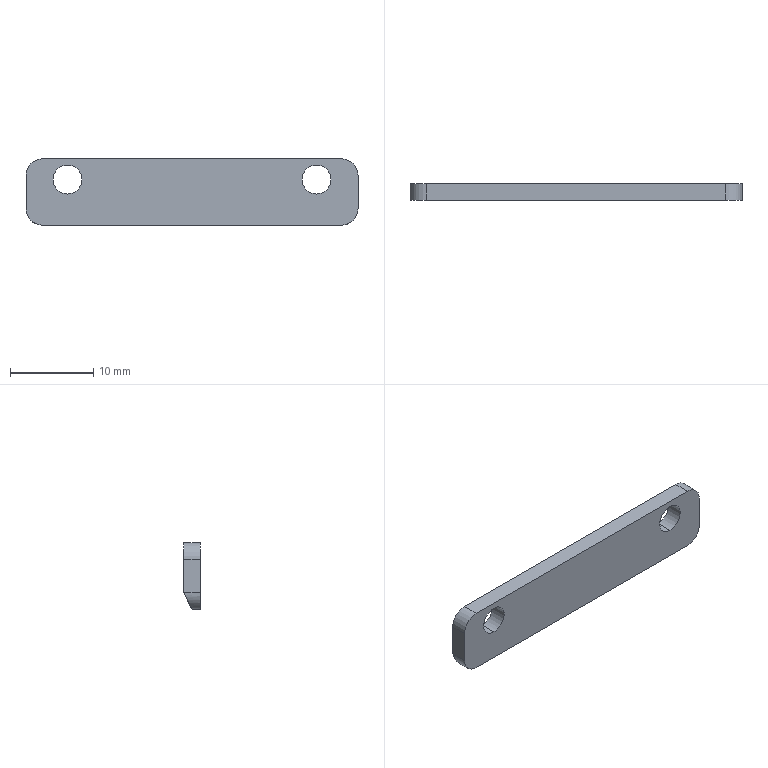Part | STEP file | 11-FG-SZ03011 | 1 solid | 15 faces | box 40 x 2 x 8 mm | volume 555.982 mm3 | cylinder 8 | plane 7 | commonest cylinder face diameters 3.5 x4 4 x4
STEP:
#1=CARTESIAN_POINT('',(-15.,1.,7.25));
#2=VERTEX_POINT('',#1);
#3=CARTESIAN_POINT('',(-15.,1.,3.75));
#4=VERTEX_POINT('',#3);
#5=CARTESIAN_POINT('',(-15.,1.,5.5));
#6=DIRECTION('',(0.,-1.,0.));
#7=DIRECTION('',(0.,0.,1.));
#8=AXIS2_PLACEMENT_3D('',#5,#6,#7);
#9=CIRCLE('',#8,1.75);
#10=EDGE_CURVE('',#2,#4,#9,.T.);
#11=ORIENTED_EDGE('',*,*,#10,.F.);
#12=CARTESIAN_POINT('',(-15.,-1.,7.25));
#13=VERTEX_POINT('',#12);
#14=CARTESIAN_POINT('',(-15.,1.,7.25));
#15=DIRECTION('',(0.,-1.,0.));
#16=VECTOR('',#15,1000.);
#17=LINE('',#14,#16);
#18=EDGE_CURVE('',#2,#13,#17,.T.);
#19=ORIENTED_EDGE('',*,*,#18,.T.);
#20=CARTESIAN_POINT('',(-15.,-1.,3.75));
#21=VERTEX_POINT('',#20);
#22=CARTESIAN_POINT('',(-15.,-1.,5.5));
#23=DIRECTION('',(0.,-1.,0.));
#24=DIRECTION('',(0.,0.,1.));
#25=AXIS2_PLACEMENT_3D('',#22,#23,#24);
#26=CIRCLE('',#25,1.75);
#27=EDGE_CURVE('',#13,#21,#26,.T.);
#28=ORIENTED_EDGE('',*,*,#27,.T.);
#29=CARTESIAN_POINT('',(-15.,1.,3.75));
#30=DIRECTION('',(0.,-1.,0.));
#31=VECTOR('',#30,1000.);
#32=LINE('',#29,#31);
#33=EDGE_CURVE('',#4,#21,#32,.T.);
#34=ORIENTED_EDGE('',*,*,#33,.F.);
#35=EDGE_LOOP('',(#11,#19,#28,#34));
#36=FACE_OUTER_BOUND('',#35,.T.);
#37=CARTESIAN_POINT('',(-15.,1.,5.5));
#38=DIRECTION('',(0.,-1.,0.));
#39=DIRECTION('',(0.,0.,-1.));
#40=AXIS2_PLACEMENT_3D('',#37,#38,#39);
#41=CYLINDRICAL_SURFACE('',#40,1.75);
#42=ADVANCED_FACE('',(#36),#41,.F.);
#43=CARTESIAN_POINT('',(15.,1.,7.25));
#44=VERTEX_POINT('',#43);
#45=CARTESIAN_POINT('',(15.,1.,3.75));
#46=VERTEX_POINT('',#45);
#47=CARTESIAN_POINT('',(15.,1.,5.5));
#48=DIRECTION('',(0.,-1.,0.));
#49=DIRECTION('',(0.,0.,-1.));
#50=AXIS2_PLACEMENT_3D('',#47,#48,#49);
#51=CIRCLE('',#50,1.75);
#52=EDGE_CURVE('',#44,#46,#51,.T.);
#53=ORIENTED_EDGE('',*,*,#52,.F.);
#54=CARTESIAN_POINT('',(15.,-1.,7.25));
#55=VERTEX_POINT('',#54);
#56=CARTESIAN_POINT('',(15.,1.,7.25));
#57=DIRECTION('',(0.,-1.,0.));
#58=VECTOR('',#57,1000.);
#59=LINE('',#56,#58);
#60=EDGE_CURVE('',#44,#55,#59,.T.);
#61=ORIENTED_EDGE('',*,*,#60,.T.);
#62=CARTESIAN_POINT('',(15.,-1.,3.75));
#63=VERTEX_POINT('',#62);
#64=CARTESIAN_POINT('',(15.,-1.,5.5));
#65=DIRECTION('',(0.,-1.,0.));
#66=DIRECTION('',(0.,0.,-1.));
#67=AXIS2_PLACEMENT_3D('',#64,#65,#66);
#68=CIRCLE('',#67,1.75);
#69=EDGE_CURVE('',#55,#63,#68,.T.);
#70=ORIENTED_EDGE('',*,*,#69,.T.);
#71=CARTESIAN_POINT('',(15.,1.,3.75));
#72=DIRECTION('',(0.,-1.,0.));
#73=VECTOR('',#72,1000.);
#74=LINE('',#71,#73);
#75=EDGE_CURVE('',#46,#63,#74,.T.);
#76=ORIENTED_EDGE('',*,*,#75,.F.);
#77=EDGE_LOOP('',(#53,#61,#70,#76));
#78=FACE_OUTER_BOUND('',#77,.T.);
#79=CARTESIAN_POINT('',(15.,1.,5.5));
#80=DIRECTION('',(0.,-1.,0.));
#81=DIRECTION('',(0.,0.,-1.));
#82=AXIS2_PLACEMENT_3D('',#79,#80,#81);
#83=CYLINDRICAL_SURFACE('',#82,1.75);
#84=ADVANCED_FACE('',(#78),#83,.F.);
#85=CARTESIAN_POINT('',(20.,1.,6.));
#86=VERTEX_POINT('',#85);
#87=CARTESIAN_POINT('',(20.,1.,2.));
#88=VERTEX_POINT('',#87);
#89=CARTESIAN_POINT('',(20.,1.,8.));
#90=DIRECTION('',(0.,0.,-1.));
#91=VECTOR('',#90,1000.);
#92=LINE('',#89,#91);
#93=EDGE_CURVE('',#86,#88,#92,.T.);
#94=ORIENTED_EDGE('',*,*,#93,.F.);
#95=CARTESIAN_POINT('',(20.,-1.,6.));
#96=VERTEX_POINT('',#95);
#97=CARTESIAN_POINT('',(20.,-1.,6.));
#98=DIRECTION('',(0.,-1.,0.));
#99=VECTOR('',#98,1000.);
#100=LINE('',#97,#99);
#101=EDGE_CURVE('',#86,#96,#100,.T.);
#102=ORIENTED_EDGE('',*,*,#101,.T.);
#103=CARTESIAN_POINT('',(20.,-1.,2.));
#104=VERTEX_POINT('',#103);
#105=CARTESIAN_POINT('',(20.,-1.,8.));
#106=DIRECTION('',(0.,0.,-1.));
#107=VECTOR('',#106,1000.);
#108=LINE('',#105,#107);
#109=EDGE_CURVE('',#96,#104,#108,.T.);
#110=ORIENTED_EDGE('',*,*,#109,.T.);
#111=CARTESIAN_POINT('',(20.,1.,2.));
#112=DIRECTION('',(0.,1.,0.));
#113=VECTOR('',#112,1000.);
#114=LINE('',#111,#113);
#115=EDGE_CURVE('',#104,#88,#114,.T.);
#116=ORIENTED_EDGE('',*,*,#115,.T.);
#117=EDGE_LOOP('',(#94,#102,#110,#116));
#118=FACE_OUTER_BOUND('',#117,.T.);
#119=CARTESIAN_POINT('',(20.,1.,8.));
#120=DIRECTION('',(-1.,0.,0.));
#121=DIRECTION('',(0.,0.,1.));
#122=AXIS2_PLACEMENT_3D('',#119,#120,#121);
#123=PLANE('',#122);
#124=ADVANCED_FACE('',(#118),#123,.F.);
#125=CARTESIAN_POINT('',(-15.,1.,5.5));
#126=DIRECTION('',(0.,-1.,0.));
#127=DIRECTION('',(0.,0.,1.));
#128=AXIS2_PLACEMENT_3D('',#125,#126,#127);
#129=CIRCLE('',#128,1.75);
#130=EDGE_CURVE('',#4,#2,#129,.T.);
#131=ORIENTED_EDGE('',*,*,#130,.T.);
#132=ORIENTED_EDGE('',*,*,#10,.T.);
#133=EDGE_LOOP('',(#131,#132));
#134=FACE_BOUND('',#133,.T.);
#135=CARTESIAN_POINT('',(15.,1.,5.5));
#136=DIRECTION('',(0.,-1.,0.));
#137=DIRECTION('',(0.,0.,-1.));
#138=AXIS2_PLACEMENT_3D('',#135,#136,#137);
#139=CIRCLE('',#138,1.75);
#140=EDGE_CURVE('',#46,#44,#139,.T.);
#141=ORIENTED_EDGE('',*,*,#140,.T.);
#142=ORIENTED_EDGE('',*,*,#52,.T.);
#143=EDGE_LOOP('',(#141,#142));
#144=FACE_BOUND('',#143,.T.);
#145=CARTESIAN_POINT('',(18.,1.,8.));
#146=VERTEX_POINT('',#145);
#147=CARTESIAN_POINT('',(-18.,1.,8.));
#148=VERTEX_POINT('',#147);
#149=CARTESIAN_POINT('',(-20.,1.,8.));
#150=DIRECTION('',(-1.,0.,0.));
#151=VECTOR('',#150,1000.);
#152=LINE('',#149,#151);
#153=EDGE_CURVE('',#146,#148,#152,.T.);
#154=ORIENTED_EDGE('',*,*,#153,.F.);
#155=CARTESIAN_POINT('',(18.,1.,6.));
#156=DIRECTION('',(0.,1.,0.));
#157=DIRECTION('',(0.,0.,-1.));
#158=AXIS2_PLACEMENT_3D('',#155,#156,#157);
#159=CIRCLE('',#158,2.);
#160=EDGE_CURVE('',#146,#86,#159,.T.);
#161=ORIENTED_EDGE('',*,*,#160,.T.);
#162=ORIENTED_EDGE('',*,*,#93,.T.);
#163=CARTESIAN_POINT('',(-20.,1.,2.));
#164=VERTEX_POINT('',#163);
#165=CARTESIAN_POINT('',(-20.,1.,2.));
#166=DIRECTION('',(1.,0.,0.));
#167=VECTOR('',#166,1000.);
#168=LINE('',#165,#167);
#169=EDGE_CURVE('',#164,#88,#168,.T.);
#170=ORIENTED_EDGE('',*,*,#169,.F.);
#171=CARTESIAN_POINT('',(-20.,1.,6.));
#172=VERTEX_POINT('',#171);
#173=CARTESIAN_POINT('',(-20.,1.,8.));
#174=DIRECTION('',(0.,0.,-1.));
#175=VECTOR('',#174,1000.);
#176=LINE('',#173,#175);
#177=EDGE_CURVE('',#172,#164,#176,.T.);
#178=ORIENTED_EDGE('',*,*,#177,.F.);
#179=CARTESIAN_POINT('',(-18.,1.,6.));
#180=DIRECTION('',(0.,1.,0.));
#181=DIRECTION('',(0.,0.,-1.));
#182=AXIS2_PLACEMENT_3D('',#179,#180,#181);
#183=CIRCLE('',#182,2.);
#184=EDGE_CURVE('',#172,#148,#183,.T.);
#185=ORIENTED_EDGE('',*,*,#184,.T.);
#186=EDGE_LOOP('',(#154,#161,#162,#170,#178,#185));
#187=FACE_OUTER_BOUND('',#186,.T.);
#188=CARTESIAN_POINT('',(-20.,1.,8.));
#189=DIRECTION('',(0.,-1.,0.));
#190=DIRECTION('',(0.,0.,-1.));
#191=AXIS2_PLACEMENT_3D('',#188,#189,#190);
#192=PLANE('',#191);
#193=ADVANCED_FACE('',(#134,#144,#187),#192,.F.);
#194=ORIENTED_EDGE('',*,*,#177,.T.);
#195=CARTESIAN_POINT('',(-20.,-1.,2.));
#196=VERTEX_POINT('',#195);
#197=CARTESIAN_POINT('',(-20.,1.,2.));
#198=DIRECTION('',(0.,-1.,0.));
#199=VECTOR('',#198,1000.);
#200=LINE('',#197,#199);
#201=EDGE_CURVE('',#164,#196,#200,.T.);
#202=ORIENTED_EDGE('',*,*,#201,.T.);
#203=CARTESIAN_POINT('',(-20.,-1.,6.));
#204=VERTEX_POINT('',#203);
#205=CARTESIAN_POINT('',(-20.,-1.,8.));
#206=DIRECTION('',(0.,0.,-1.));
#207=VECTOR('',#206,1000.);
#208=LINE('',#205,#207);
#209=EDGE_CURVE('',#204,#196,#208,.T.);
#210=ORIENTED_EDGE('',*,*,#209,.F.);
#211=CARTESIAN_POINT('',(-20.,1.,6.));
#212=DIRECTION('',(0.,1.,0.));
#213=VECTOR('',#212,1000.);
#214=LINE('',#211,#213);
#215=EDGE_CURVE('',#204,#172,#214,.T.);
#216=ORIENTED_EDGE('',*,*,#215,.T.);
#217=EDGE_LOOP('',(#194,#202,#210,#216));
#218=FACE_OUTER_BOUND('',#217,.T.);
#219=CARTESIAN_POINT('',(-20.,1.,8.));
#220=DIRECTION('',(1.,0.,0.));
#221=DIRECTION('',(0.,0.,-1.));
#222=AXIS2_PLACEMENT_3D('',#219,#220,#221);
#223=PLANE('',#222);
#224=ADVANCED_FACE('',(#218),#223,.F.);
#225=CARTESIAN_POINT('',(-15.,-1.,5.5));
#226=DIRECTION('',(0.,-1.,0.));
#227=DIRECTION('',(0.,0.,1.));
#228=AXIS2_PLACEMENT_3D('',#225,#226,#227);
#229=CIRCLE('',#228,1.75);
#230=EDGE_CURVE('',#21,#13,#229,.T.);
#231=ORIENTED_EDGE('',*,*,#230,.F.);
#232=ORIENTED_EDGE('',*,*,#27,.F.);
#233=EDGE_LOOP('',(#231,#232));
#234=FACE_BOUND('',#233,.T.);
#235=CARTESIAN_POINT('',(15.,-1.,5.5));
#236=DIRECTION('',(0.,-1.,0.));
#237=DIRECTION('',(0.,0.,-1.));
#238=AXIS2_PLACEMENT_3D('',#235,#236,#237);
#239=CIRCLE('',#238,1.75);
#240=EDGE_CURVE('',#63,#55,#239,.T.);
#241=ORIENTED_EDGE('',*,*,#240,.F.);
#242=ORIENTED_EDGE('',*,*,#69,.F.);
#243=EDGE_LOOP('',(#241,#242));
#244=FACE_BOUND('',#243,.T.);
#245=ORIENTED_EDGE('',*,*,#109,.F.);
#246=CARTESIAN_POINT('',(18.,-1.,8.));
#247=VERTEX_POINT('',#246);
#248=CARTESIAN_POINT('',(18.,-1.,6.));
#249=DIRECTION('',(0.,-1.,0.));
#250=DIRECTION('',(0.,0.,1.));
#251=AXIS2_PLACEMENT_3D('',#248,#249,#250);
#252=CIRCLE('',#251,2.);
#253=EDGE_CURVE('',#96,#247,#252,.T.);
#254=ORIENTED_EDGE('',*,*,#253,.T.);
#255=CARTESIAN_POINT('',(-18.,-1.,8.));
#256=VERTEX_POINT('',#255);
#257=CARTESIAN_POINT('',(-20.,-1.,8.));
#258=DIRECTION('',(1.,0.,0.));
#259=VECTOR('',#258,1000.);
#260=LINE('',#257,#259);
#261=EDGE_CURVE('',#256,#247,#260,.T.);
#262=ORIENTED_EDGE('',*,*,#261,.F.);
#263=CARTESIAN_POINT('',(-18.,-1.,6.));
#264=DIRECTION('',(0.,-1.,0.));
#265=DIRECTION('',(0.,0.,1.));
#266=AXIS2_PLACEMENT_3D('',#263,#264,#265);
#267=CIRCLE('',#266,2.);
#268=EDGE_CURVE('',#256,#204,#267,.T.);
#269=ORIENTED_EDGE('',*,*,#268,.T.);
#270=ORIENTED_EDGE('',*,*,#209,.T.);
#271=CARTESIAN_POINT('',(-18.,-1.,0.));
#272=VERTEX_POINT('',#271);
#273=CARTESIAN_POINT('',(-18.,-1.,2.));
#274=DIRECTION('',(0.,-1.,0.));
#275=DIRECTION('',(0.,0.,1.));
#276=AXIS2_PLACEMENT_3D('',#273,#274,#275);
#277=CIRCLE('',#276,2.);
#278=EDGE_CURVE('',#196,#272,#277,.T.);
#279=ORIENTED_EDGE('',*,*,#278,.T.);
#280=CARTESIAN_POINT('',(18.,-1.,0.));
#281=VERTEX_POINT('',#280);
#282=CARTESIAN_POINT('',(-20.,-1.,0.));
#283=DIRECTION('',(1.,0.,0.));
#284=VECTOR('',#283,1000.);
#285=LINE('',#282,#284);
#286=EDGE_CURVE('',#272,#281,#285,.T.);
#287=ORIENTED_EDGE('',*,*,#286,.T.);
#288=CARTESIAN_POINT('',(18.,-1.,2.));
#289=DIRECTION('',(0.,-1.,0.));
#290=DIRECTION('',(0.,0.,1.));
#291=AXIS2_PLACEMENT_3D('',#288,#289,#290);
#292=CIRCLE('',#291,2.);
#293=EDGE_CURVE('',#281,#104,#292,.T.);
#294=ORIENTED_EDGE('',*,*,#293,.T.);
#295=EDGE_LOOP('',(#245,#254,#262,#269,#270,#279,#287,#294));
#296=FACE_OUTER_BOUND('',#295,.T.);
#297=CARTESIAN_POINT('',(-20.,-1.,8.));
#298=DIRECTION('',(0.,1.,0.));
#299=DIRECTION('',(0.,0.,1.));
#300=AXIS2_PLACEMENT_3D('',#297,#298,#299);
#301=PLANE('',#300);
#302=ADVANCED_FACE('',(#234,#244,#296),#301,.F.);
#303=ORIENTED_EDGE('',*,*,#261,.T.);
#304=CARTESIAN_POINT('',(18.,1.,8.));
#305=DIRECTION('',(0.,1.,0.));
#306=VECTOR('',#305,1000.);
#307=LINE('',#304,#306);
#308=EDGE_CURVE('',#247,#146,#307,.T.);
#309=ORIENTED_EDGE('',*,*,#308,.T.);
#310=ORIENTED_EDGE('',*,*,#153,.T.);
#311=CARTESIAN_POINT('',(-18.,-1.,8.));
#312=DIRECTION('',(0.,-1.,0.));
#313=VECTOR('',#312,1000.);
#314=LINE('',#311,#313);
#315=EDGE_CURVE('',#148,#256,#314,.T.);
#316=ORIENTED_EDGE('',*,*,#315,.T.);
#317=EDGE_LOOP('',(#303,#309,#310,#316));
#318=FACE_OUTER_BOUND('',#317,.T.);
#319=CARTESIAN_POINT('',(0.,0.,8.));
#320=DIRECTION('',(0.,0.,1.));
#321=DIRECTION('',(1.,0.,0.));
#322=AXIS2_PLACEMENT_3D('',#319,#320,#321);
#323=PLANE('',#322);
#324=ADVANCED_FACE('',(#318),#323,.T.);
#325=CARTESIAN_POINT('',(-18.,0.,0.));
#326=VERTEX_POINT('',#325);
#327=CARTESIAN_POINT('',(18.,0.,0.));
#328=VERTEX_POINT('',#327);
#329=CARTESIAN_POINT('',(-20.,0.,0.));
#330=DIRECTION('',(1.,0.,0.));
#331=VECTOR('',#330,1000.);
#332=LINE('',#329,#331);
#333=EDGE_CURVE('',#326,#328,#332,.T.);
#334=ORIENTED_EDGE('',*,*,#333,.T.);
#335=CARTESIAN_POINT('',(18.,0.,0.));
#336=DIRECTION('',(0.,-1.,0.));
#337=VECTOR('',#336,1000.);
#338=LINE('',#335,#337);
#339=EDGE_CURVE('',#328,#281,#338,.T.);
#340=ORIENTED_EDGE('',*,*,#339,.T.);
#341=ORIENTED_EDGE('',*,*,#286,.F.);
#342=CARTESIAN_POINT('',(-18.,0.,0.));
#343=DIRECTION('',(0.,1.,0.));
#344=VECTOR('',#343,1000.);
#345=LINE('',#342,#344);
#346=EDGE_CURVE('',#272,#326,#345,.T.);
#347=ORIENTED_EDGE('',*,*,#346,.T.);
#348=EDGE_LOOP('',(#334,#340,#341,#347));
#349=FACE_OUTER_BOUND('',#348,.T.);
#350=CARTESIAN_POINT('',(0.,0.,0.));
#351=DIRECTION('',(0.,0.,1.));
#352=DIRECTION('',(1.,0.,0.));
#353=AXIS2_PLACEMENT_3D('',#350,#351,#352);
#354=PLANE('',#353);
#355=ADVANCED_FACE('',(#349),#354,.F.);
#356=ORIENTED_EDGE('',*,*,#60,.F.);
#357=ORIENTED_EDGE('',*,*,#140,.F.);
#358=ORIENTED_EDGE('',*,*,#75,.T.);
#359=ORIENTED_EDGE('',*,*,#240,.T.);
#360=EDGE_LOOP('',(#356,#357,#358,#359));
#361=FACE_OUTER_BOUND('',#360,.T.);
#362=CARTESIAN_POINT('',(15.,1.,5.5));
#363=DIRECTION('',(0.,-1.,0.));
#364=DIRECTION('',(0.,0.,-1.));
#365=AXIS2_PLACEMENT_3D('',#362,#363,#364);
#366=CYLINDRICAL_SURFACE('',#365,1.75);
#367=ADVANCED_FACE('',(#361),#366,.F.);
#368=ORIENTED_EDGE('',*,*,#18,.F.);
#369=ORIENTED_EDGE('',*,*,#130,.F.);
#370=ORIENTED_EDGE('',*,*,#33,.T.);
#371=ORIENTED_EDGE('',*,*,#230,.T.);
#372=EDGE_LOOP('',(#368,#369,#370,#371));
#373=FACE_OUTER_BOUND('',#372,.T.);
#374=CARTESIAN_POINT('',(-15.,1.,5.5));
#375=DIRECTION('',(0.,-1.,0.));
#376=DIRECTION('',(0.,0.,-1.));
#377=AXIS2_PLACEMENT_3D('',#374,#375,#376);
#378=CYLINDRICAL_SURFACE('',#377,1.75);
#379=ADVANCED_FACE('',(#373),#378,.F.);
#380=ORIENTED_EDGE('',*,*,#169,.T.);
#381=CARTESIAN_POINT('',(20.,1.,2.));
#382=CARTESIAN_POINT('',(20.,0.4142,0.8284));
#383=CARTESIAN_POINT('',(19.172,0.,0.));
#384=CARTESIAN_POINT('',(18.,0.,0.));
#385=(BOUNDED_CURVE()B_SPLINE_CURVE(3,(#381,#382,#383,#384),.UNSPECIFIED.,.F.,.F.)B_SPLINE_CURVE_WITH_KNOTS((4,4),(1.571,3.142),.UNSPECIFIED.)CURVE()GEOMETRIC_REPRESENTATION_ITEM()RATIONAL_B_SPLINE_CURVE((1.,0.8047,0.8047,1.))REPRESENTATION_ITEM(''));
#386=EDGE_CURVE('',#88,#328,#385,.T.);
#387=ORIENTED_EDGE('',*,*,#386,.T.);
#388=ORIENTED_EDGE('',*,*,#333,.F.);
#389=CARTESIAN_POINT('',(-18.,0.,0.));
#390=CARTESIAN_POINT('',(-19.172,0.,0.));
#391=CARTESIAN_POINT('',(-20.,0.4142,0.8284));
#392=CARTESIAN_POINT('',(-20.,1.,2.));
#393=(BOUNDED_CURVE()B_SPLINE_CURVE(3,(#389,#390,#391,#392),.UNSPECIFIED.,.F.,.F.)B_SPLINE_CURVE_WITH_KNOTS((4,4),(0.,1.571),.UNSPECIFIED.)CURVE()GEOMETRIC_REPRESENTATION_ITEM()RATIONAL_B_SPLINE_CURVE((1.,0.8047,0.8047,1.))REPRESENTATION_ITEM(''));
#394=EDGE_CURVE('',#326,#164,#393,.T.);
#395=ORIENTED_EDGE('',*,*,#394,.T.);
#396=EDGE_LOOP('',(#380,#387,#388,#395));
#397=FACE_OUTER_BOUND('',#396,.T.);
#398=CARTESIAN_POINT('',(-20.,1.,2.));
#399=DIRECTION('',(0.,-0.8944,0.4472));
#400=DIRECTION('',(0.,-0.4472,-0.8944));
#401=AXIS2_PLACEMENT_3D('',#398,#399,#400);
#402=PLANE('',#401);
#403=ADVANCED_FACE('',(#397),#402,.F.);
#404=ORIENTED_EDGE('',*,*,#253,.F.);
#405=ORIENTED_EDGE('',*,*,#101,.F.);
#406=ORIENTED_EDGE('',*,*,#160,.F.);
#407=ORIENTED_EDGE('',*,*,#308,.F.);
#408=EDGE_LOOP('',(#404,#405,#406,#407));
#409=FACE_OUTER_BOUND('',#408,.T.);
#410=CARTESIAN_POINT('',(18.,0.,6.));
#411=DIRECTION('',(0.,-1.,0.));
#412=DIRECTION('',(0.,0.,-1.));
#413=AXIS2_PLACEMENT_3D('',#410,#411,#412);
#414=CYLINDRICAL_SURFACE('',#413,2.);
#415=ADVANCED_FACE('',(#409),#414,.T.);
#416=ORIENTED_EDGE('',*,*,#293,.F.);
#417=ORIENTED_EDGE('',*,*,#339,.F.);
#418=ORIENTED_EDGE('',*,*,#386,.F.);
#419=ORIENTED_EDGE('',*,*,#115,.F.);
#420=EDGE_LOOP('',(#416,#417,#418,#419));
#421=FACE_OUTER_BOUND('',#420,.T.);
#422=CARTESIAN_POINT('',(18.,1.,2.));
#423=DIRECTION('',(0.,1.,0.));
#424=DIRECTION('',(0.,0.,1.));
#425=AXIS2_PLACEMENT_3D('',#422,#423,#424);
#426=CYLINDRICAL_SURFACE('',#425,2.);
#427=ADVANCED_FACE('',(#421),#426,.T.);
#428=ORIENTED_EDGE('',*,*,#394,.F.);
#429=ORIENTED_EDGE('',*,*,#346,.F.);
#430=ORIENTED_EDGE('',*,*,#278,.F.);
#431=ORIENTED_EDGE('',*,*,#201,.F.);
#432=EDGE_LOOP('',(#428,#429,#430,#431));
#433=FACE_OUTER_BOUND('',#432,.T.);
#434=CARTESIAN_POINT('',(-18.,1.,2.));
#435=DIRECTION('',(0.,-1.,0.));
#436=DIRECTION('',(0.,0.,-1.));
#437=AXIS2_PLACEMENT_3D('',#434,#435,#436);
#438=CYLINDRICAL_SURFACE('',#437,2.);
#439=ADVANCED_FACE('',(#433),#438,.T.);
#440=ORIENTED_EDGE('',*,*,#184,.F.);
#441=ORIENTED_EDGE('',*,*,#215,.F.);
#442=ORIENTED_EDGE('',*,*,#268,.F.);
#443=ORIENTED_EDGE('',*,*,#315,.F.);
#444=EDGE_LOOP('',(#440,#441,#442,#443));
#445=FACE_OUTER_BOUND('',#444,.T.);
#446=CARTESIAN_POINT('',(-18.,0.,6.));
#447=DIRECTION('',(0.,1.,0.));
#448=DIRECTION('',(0.,0.,1.));
#449=AXIS2_PLACEMENT_3D('',#446,#447,#448);
#450=CYLINDRICAL_SURFACE('',#449,2.);
#451=ADVANCED_FACE('',(#445),#450,.T.);
#452=CLOSED_SHELL('',(#42,#84,#124,#193,#224,#302,#324,#355,#367,#379,#403,#415,#427,#439,#451));
#453=MANIFOLD_SOLID_BREP('',#452);
#454=CARTESIAN_POINT('',(0.,0.,0.));
#455=DIRECTION('',(0.,0.,1.));
#456=DIRECTION('',(1.,0.,0.));
#457=AXIS2_PLACEMENT_3D('',#454,#455,#456);
#458=(LENGTH_UNIT()NAMED_UNIT(*)SI_UNIT(.MILLI.,.METRE.));
#459=UNCERTAINTY_MEASURE_WITH_UNIT(LENGTH_MEASURE(0.00001),#458,'','');
#460=(NAMED_UNIT(*)PLANE_ANGLE_UNIT()SI_UNIT($,.RADIAN.));
#461=(NAMED_UNIT(*)SI_UNIT($,.STERADIAN.)SOLID_ANGLE_UNIT());
#462=(GEOMETRIC_REPRESENTATION_CONTEXT(3)GLOBAL_UNCERTAINTY_ASSIGNED_CONTEXT((#459))GLOBAL_UNIT_ASSIGNED_CONTEXT((#458,#460,#461))REPRESENTATION_CONTEXT('',''));
#463=ADVANCED_BREP_SHAPE_REPRESENTATION('',(#453,#457),#462);